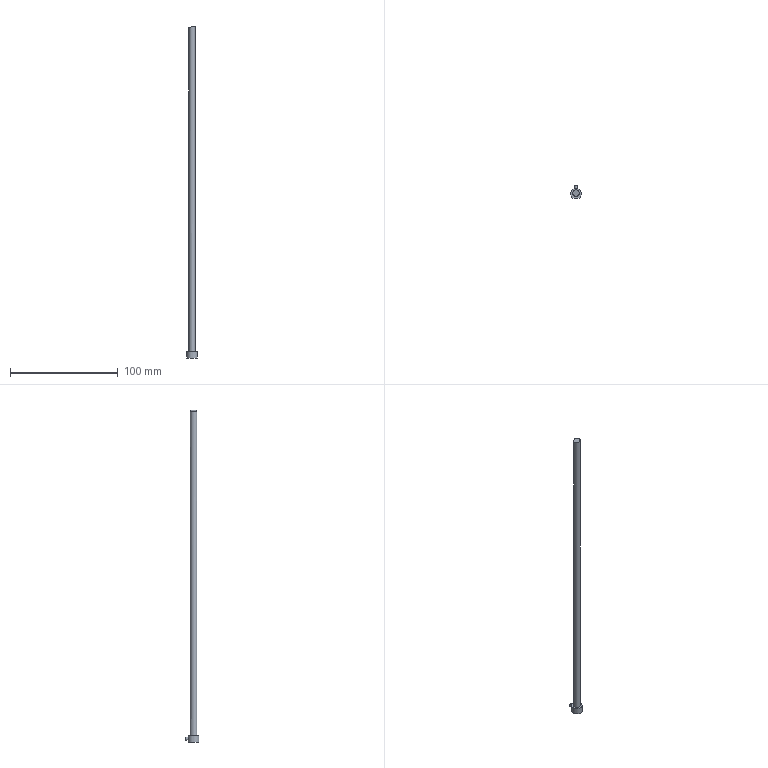Part | STEP file | E106-21-315 | 1 solid | 8 faces | box 10 x 13 x 308.066 mm | volume 9009 mm3 | cylinder 3 | plane 3 | spline 1 | cone 1 | commonest cylinder face diameters 3 x1 6 x1 10 x1